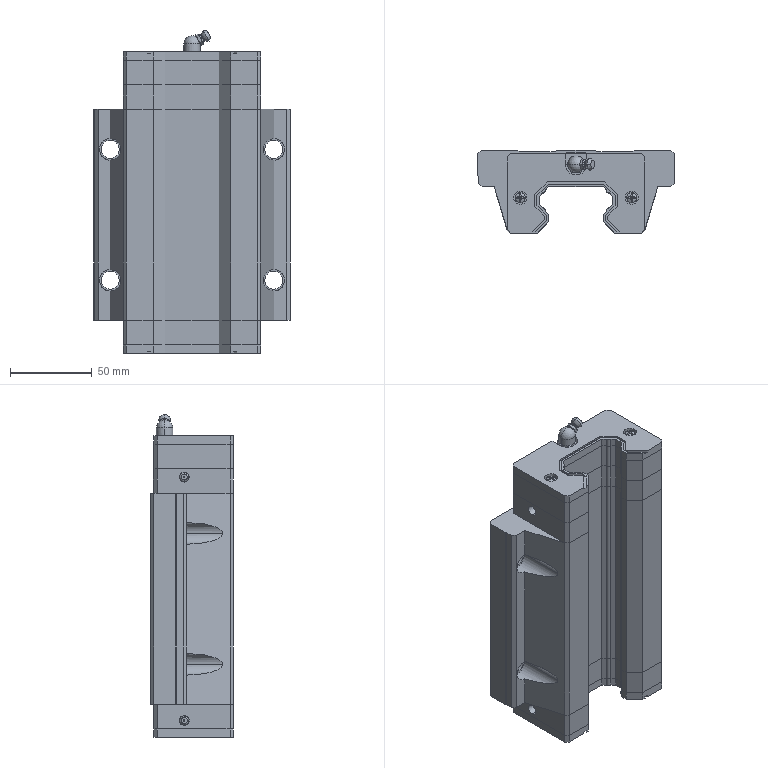Part | SolidWorks | features ICE 22, Extrusion 5, MirrorPattern 5, Fillet 4, MirrorSolid 4, Chamfer 3, RevCut 3, Dome 2, LPattern 2, Revolution 2, CreateAssemFeat 1, DeleteBody 1, LibraryFeature 1 | 7 solids | 475 faces | box 120 x 50.5 x 197.1 mm | volume 674621 mm3 | plane 323 | cylinder 94 | torus 25 | cone 23 | sphere 10 | commonest cylinder face diameters 3.924 x36 6.06 x12 0.818 x8 6.384 x8 7.98 x8 11 x8